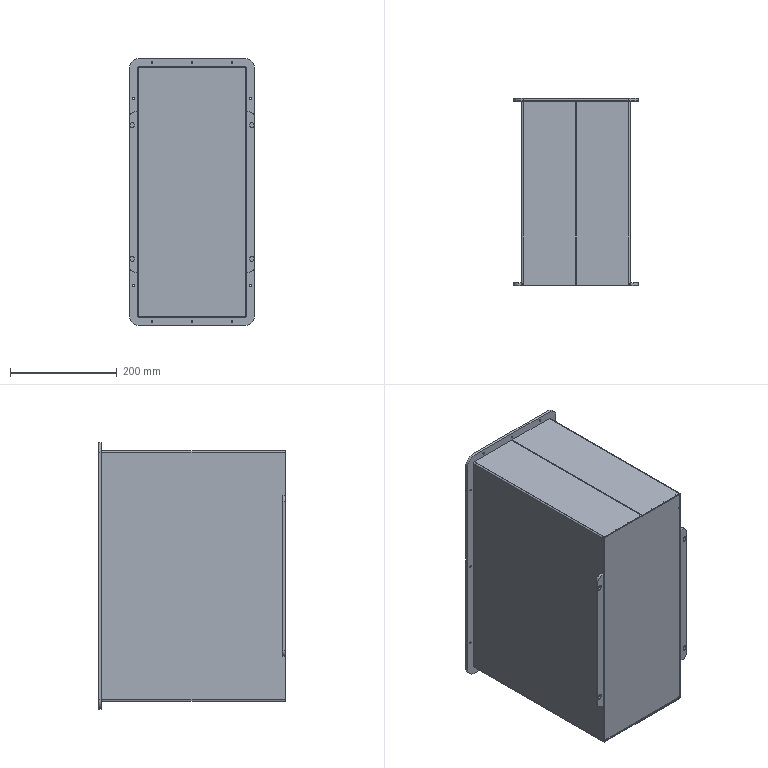Part | SolidWorks | features HoleWzd 4, ICE 4, 3DProfileFeature 3, Fillet 2, CosmeticWeldCutList 1, EdgeFlange 1, FlatPattern 1, SMBaseFlange 1, SheetMetal 1 | 5 solids | 126 faces | box 234 x 350 x 500 mm | volume 1268119 mm3 | plane 66 | cylinder 60 | commonest cylinder face diameters 3.3 x24 7 x12 2 x8 6 x8 20 x4 36 x4